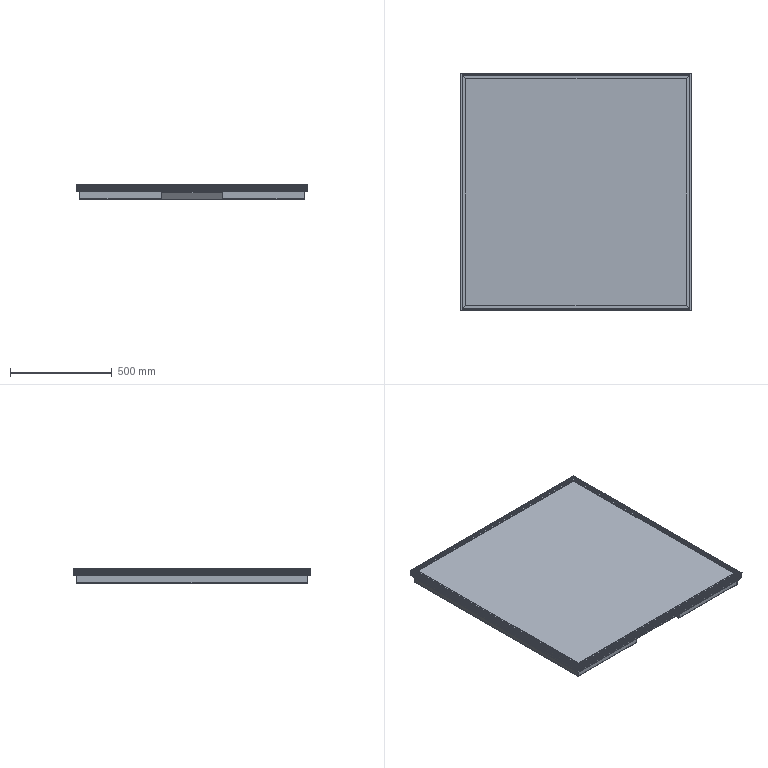Part | 7 solids | 478 faces | box 1140 x 1170 x 70 mm | volume 23307556 mm3 | plane 328 | cylinder 138 | spline 12 | commonest cylinder face diameters 7 x50 0.4 x37 2 x16 14 x14 2.4 x11 1 x8